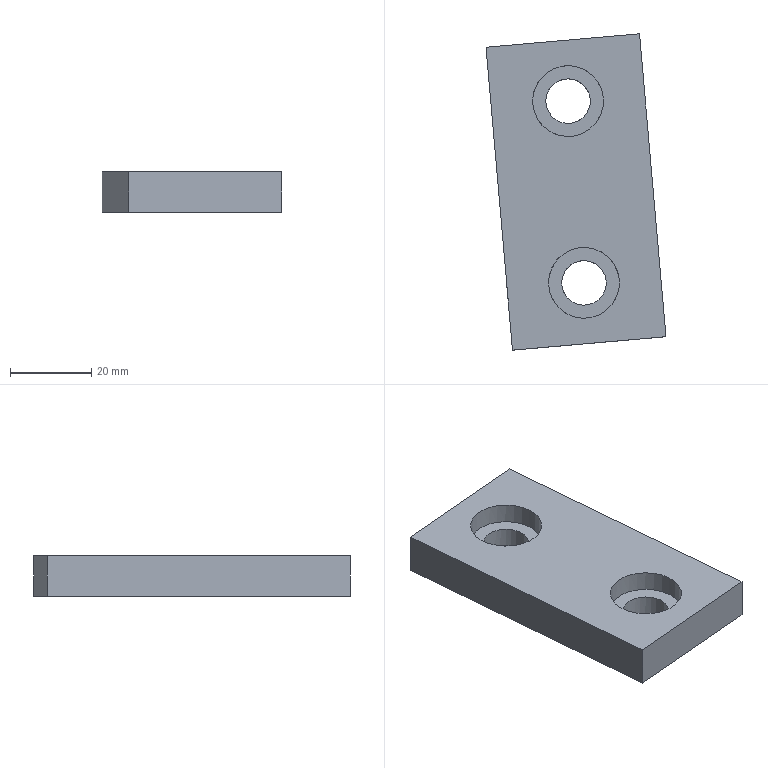Part | NX | features solid 2 | 1 solid | 12 faces | box 44.392 x 78.027 x 10 mm | volume 25144 mm3 | plane 8 | cylinder 4 | commonest cylinder face diameters 11 x2 17.5 x2
STEP:
#1=CARTESIAN_POINT('',(788.744,651.222,-208.));
#2=VERTEX_POINT('',#1);
#3=CARTESIAN_POINT('',(788.744,651.222,-218.));
#4=VERTEX_POINT('',#3);
#5=CARTESIAN_POINT('',(788.744,651.222,-208.));
#6=DIRECTION('',(0.,0.,-1.));
#7=VECTOR('',#6,1000.);
#8=LINE('',#5,#7);
#9=EDGE_CURVE('',#2,#4,#8,.T.);
#10=ORIENTED_EDGE('',*,*,#9,.F.);
#11=CARTESIAN_POINT('',(750.888,647.91,-208.));
#12=VERTEX_POINT('',#11);
#13=CARTESIAN_POINT('',(769.816,649.566,-208.));
#14=DIRECTION('',(0.9962,0.08716,0.));
#15=VECTOR('',#14,1000.);
#16=LINE('',#13,#15);
#17=EDGE_CURVE('',#12,#2,#16,.T.);
#18=ORIENTED_EDGE('',*,*,#17,.F.);
#19=CARTESIAN_POINT('',(750.888,647.91,-218.));
#20=VERTEX_POINT('',#19);
#21=CARTESIAN_POINT('',(750.888,647.91,-208.));
#22=DIRECTION('',(0.,0.,1.));
#23=VECTOR('',#22,1000.);
#24=LINE('',#21,#23);
#25=EDGE_CURVE('',#20,#12,#24,.T.);
#26=ORIENTED_EDGE('',*,*,#25,.F.);
#27=CARTESIAN_POINT('',(769.816,649.566,-218.));
#28=DIRECTION('',(-0.9962,-0.08716,0.));
#29=VECTOR('',#28,1000.);
#30=LINE('',#27,#29);
#31=EDGE_CURVE('',#4,#20,#30,.T.);
#32=ORIENTED_EDGE('',*,*,#31,.F.);
#33=EDGE_LOOP('',(#10,#18,#26,#32));
#34=FACE_BOUND('',#33,.T.);
#35=CARTESIAN_POINT('',(769.816,649.566,-208.));
#36=DIRECTION('',(0.08716,-0.9962,0.));
#37=DIRECTION('',(0.,0.,1.));
#38=AXIS2_PLACEMENT_3D('',#35,#36,#37);
#39=PLANE('',#38);
#40=ADVANCED_FACE('',(#34),#39,.T.);
#41=CARTESIAN_POINT('',(782.207,725.936,-208.));
#42=VERTEX_POINT('',#41);
#43=CARTESIAN_POINT('',(782.207,725.936,-208.));
#44=DIRECTION('',(0.08716,-0.9962,0.));
#45=VECTOR('',#44,1000.);
#46=LINE('',#43,#45);
#47=EDGE_CURVE('',#42,#2,#46,.T.);
#48=ORIENTED_EDGE('',*,*,#47,.T.);
#49=ORIENTED_EDGE('',*,*,#9,.T.);
#50=CARTESIAN_POINT('',(782.207,725.936,-218.));
#51=VERTEX_POINT('',#50);
#52=CARTESIAN_POINT('',(782.207,725.936,-218.));
#53=DIRECTION('',(0.08716,-0.9962,0.));
#54=VECTOR('',#53,1000.);
#55=LINE('',#52,#54);
#56=EDGE_CURVE('',#51,#4,#55,.T.);
#57=ORIENTED_EDGE('',*,*,#56,.F.);
#58=CARTESIAN_POINT('',(782.207,725.936,-208.));
#59=DIRECTION('',(0.,0.,1.));
#60=VECTOR('',#59,1000.);
#61=LINE('',#58,#60);
#62=EDGE_CURVE('',#51,#42,#61,.T.);
#63=ORIENTED_EDGE('',*,*,#62,.T.);
#64=EDGE_LOOP('',(#48,#49,#57,#63));
#65=FACE_BOUND('',#64,.T.);
#66=CARTESIAN_POINT('',(782.207,725.936,-208.));
#67=DIRECTION('',(0.9962,0.08716,0.));
#68=DIRECTION('',(-0.08716,0.9962,0.));
#69=AXIS2_PLACEMENT_3D('',#66,#67,#68);
#70=PLANE('',#69);
#71=ADVANCED_FACE('',(#65),#70,.T.);
#72=CARTESIAN_POINT('',(770.066,709.817,-218.));
#73=VERTEX_POINT('',#72);
#74=CARTESIAN_POINT('',(764.587,709.337,-218.));
#75=DIRECTION('',(0.,0.,1.));
#76=DIRECTION('',(0.9962,0.08716,0.));
#77=AXIS2_PLACEMENT_3D('',#74,#75,#76);
#78=CIRCLE('',#77,5.5);
#79=EDGE_CURVE('',#73,#73,#78,.T.);
#80=ORIENTED_EDGE('',*,*,#79,.T.);
#81=EDGE_LOOP('',(#80));
#82=FACE_BOUND('',#81,.T.);
#83=CARTESIAN_POINT('',(773.988,664.988,-218.));
#84=VERTEX_POINT('',#83);
#85=CARTESIAN_POINT('',(768.509,664.509,-218.));
#86=DIRECTION('',(0.,0.,1.));
#87=DIRECTION('',(0.9962,0.08716,0.));
#88=AXIS2_PLACEMENT_3D('',#85,#86,#87);
#89=CIRCLE('',#88,5.5);
#90=EDGE_CURVE('',#84,#84,#89,.T.);
#91=ORIENTED_EDGE('',*,*,#90,.T.);
#92=EDGE_LOOP('',(#91));
#93=FACE_BOUND('',#92,.T.);
#94=ORIENTED_EDGE('',*,*,#56,.T.);
#95=ORIENTED_EDGE('',*,*,#31,.T.);
#96=CARTESIAN_POINT('',(744.352,722.624,-218.));
#97=VERTEX_POINT('',#96);
#98=CARTESIAN_POINT('',(744.352,722.624,-218.));
#99=DIRECTION('',(0.08716,-0.9962,0.));
#100=VECTOR('',#99,1000.);
#101=LINE('',#98,#100);
#102=EDGE_CURVE('',#97,#20,#101,.T.);
#103=ORIENTED_EDGE('',*,*,#102,.F.);
#104=CARTESIAN_POINT('',(763.279,724.28,-218.));
#105=DIRECTION('',(0.9962,0.08716,0.));
#106=VECTOR('',#105,1000.);
#107=LINE('',#104,#106);
#108=EDGE_CURVE('',#97,#51,#107,.T.);
#109=ORIENTED_EDGE('',*,*,#108,.T.);
#110=EDGE_LOOP('',(#94,#95,#103,#109));
#111=FACE_BOUND('',#110,.T.);
#112=CARTESIAN_POINT('',(763.279,724.28,-218.));
#113=DIRECTION('',(0.,0.,-1.));
#114=DIRECTION('',(0.08716,-0.9962,0.));
#115=AXIS2_PLACEMENT_3D('',#112,#113,#114);
#116=PLANE('',#115);
#117=ADVANCED_FACE('',(#82,#93,#111),#116,.T.);
#118=ORIENTED_EDGE('',*,*,#102,.T.);
#119=ORIENTED_EDGE('',*,*,#25,.T.);
#120=CARTESIAN_POINT('',(744.352,722.624,-208.));
#121=VERTEX_POINT('',#120);
#122=CARTESIAN_POINT('',(744.352,722.624,-208.));
#123=DIRECTION('',(0.08716,-0.9962,0.));
#124=VECTOR('',#123,1000.);
#125=LINE('',#122,#124);
#126=EDGE_CURVE('',#121,#12,#125,.T.);
#127=ORIENTED_EDGE('',*,*,#126,.F.);
#128=CARTESIAN_POINT('',(744.352,722.624,-208.));
#129=DIRECTION('',(0.,0.,-1.));
#130=VECTOR('',#129,1000.);
#131=LINE('',#128,#130);
#132=EDGE_CURVE('',#121,#97,#131,.T.);
#133=ORIENTED_EDGE('',*,*,#132,.T.);
#134=EDGE_LOOP('',(#118,#119,#127,#133));
#135=FACE_BOUND('',#134,.T.);
#136=CARTESIAN_POINT('',(744.352,722.624,-208.));
#137=DIRECTION('',(-0.9962,-0.08716,0.));
#138=DIRECTION('',(0.08716,-0.9962,0.));
#139=AXIS2_PLACEMENT_3D('',#136,#137,#138);
#140=PLANE('',#139);
#141=ADVANCED_FACE('',(#135),#140,.T.);
#142=CARTESIAN_POINT('',(763.279,724.28,-208.));
#143=DIRECTION('',(-0.9962,-0.08716,0.));
#144=VECTOR('',#143,1000.);
#145=LINE('',#142,#144);
#146=EDGE_CURVE('',#42,#121,#145,.T.);
#147=ORIENTED_EDGE('',*,*,#146,.F.);
#148=ORIENTED_EDGE('',*,*,#62,.F.);
#149=ORIENTED_EDGE('',*,*,#108,.F.);
#150=ORIENTED_EDGE('',*,*,#132,.F.);
#151=EDGE_LOOP('',(#147,#148,#149,#150));
#152=FACE_BOUND('',#151,.T.);
#153=CARTESIAN_POINT('',(763.279,724.28,-208.));
#154=DIRECTION('',(-0.08716,0.9962,0.));
#155=DIRECTION('',(0.,0.,-1.));
#156=AXIS2_PLACEMENT_3D('',#153,#154,#155);
#157=PLANE('',#156);
#158=ADVANCED_FACE('',(#152),#157,.T.);
#159=CARTESIAN_POINT('',(755.837,709.337,-208.));
#160=VERTEX_POINT('',#159);
#161=CARTESIAN_POINT('',(764.587,709.337,-208.));
#162=DIRECTION('',(0.,0.,-1.));
#163=DIRECTION('',(-1.,0.,0.));
#164=AXIS2_PLACEMENT_3D('',#161,#162,#163);
#165=CIRCLE('',#164,8.75);
#166=EDGE_CURVE('',#160,#160,#165,.T.);
#167=ORIENTED_EDGE('',*,*,#166,.T.);
#168=EDGE_LOOP('',(#167));
#169=FACE_BOUND('',#168,.T.);
#170=CARTESIAN_POINT('',(759.759,664.509,-208.));
#171=VERTEX_POINT('',#170);
#172=CARTESIAN_POINT('',(768.509,664.509,-208.));
#173=DIRECTION('',(0.,0.,-1.));
#174=DIRECTION('',(-1.,0.,0.));
#175=AXIS2_PLACEMENT_3D('',#172,#173,#174);
#176=CIRCLE('',#175,8.75);
#177=EDGE_CURVE('',#171,#171,#176,.T.);
#178=ORIENTED_EDGE('',*,*,#177,.T.);
#179=EDGE_LOOP('',(#178));
#180=FACE_BOUND('',#179,.T.);
#181=ORIENTED_EDGE('',*,*,#146,.T.);
#182=ORIENTED_EDGE('',*,*,#126,.T.);
#183=ORIENTED_EDGE('',*,*,#17,.T.);
#184=ORIENTED_EDGE('',*,*,#47,.F.);
#185=EDGE_LOOP('',(#181,#182,#183,#184));
#186=FACE_BOUND('',#185,.T.);
#187=CARTESIAN_POINT('',(763.279,724.28,-208.));
#188=DIRECTION('',(0.,0.,1.));
#189=DIRECTION('',(-0.08716,0.9962,0.));
#190=AXIS2_PLACEMENT_3D('',#187,#188,#189);
#191=PLANE('',#190);
#192=ADVANCED_FACE('',(#169,#180,#186),#191,.T.);
#193=CARTESIAN_POINT('',(763.009,664.509,-213.));
#194=VERTEX_POINT('',#193);
#195=CARTESIAN_POINT('',(768.509,664.509,-213.));
#196=DIRECTION('',(0.,0.,-1.));
#197=DIRECTION('',(-1.,0.,0.));
#198=AXIS2_PLACEMENT_3D('',#195,#196,#197);
#199=CIRCLE('',#198,5.5);
#200=EDGE_CURVE('',#194,#194,#199,.F.);
#201=ORIENTED_EDGE('',*,*,#200,.T.);
#202=EDGE_LOOP('',(#201));
#203=FACE_BOUND('',#202,.T.);
#204=ORIENTED_EDGE('',*,*,#90,.F.);
#205=EDGE_LOOP('',(#204));
#206=FACE_BOUND('',#205,.T.);
#207=CARTESIAN_POINT('',(768.509,664.509,-218.));
#208=DIRECTION('',(0.,0.,1.));
#209=DIRECTION('',(0.9962,0.08716,0.));
#210=AXIS2_PLACEMENT_3D('',#207,#208,#209);
#211=CYLINDRICAL_SURFACE('',#210,5.5);
#212=ADVANCED_FACE('',(#203,#206),#211,.F.);
#213=CARTESIAN_POINT('',(777.225,665.271,-213.));
#214=VERTEX_POINT('',#213);
#215=CARTESIAN_POINT('',(768.509,664.509,-213.));
#216=DIRECTION('',(0.,0.,1.));
#217=DIRECTION('',(0.9962,0.08716,0.));
#218=AXIS2_PLACEMENT_3D('',#215,#216,#217);
#219=CIRCLE('',#218,8.75);
#220=EDGE_CURVE('',#214,#214,#219,.T.);
#221=ORIENTED_EDGE('',*,*,#220,.T.);
#222=EDGE_LOOP('',(#221));
#223=FACE_BOUND('',#222,.T.);
#224=ORIENTED_EDGE('',*,*,#200,.F.);
#225=EDGE_LOOP('',(#224));
#226=FACE_BOUND('',#225,.T.);
#227=CARTESIAN_POINT('',(768.509,664.509,-213.));
#228=DIRECTION('',(0.,0.,-1.));
#229=DIRECTION('',(-0.9962,-0.08716,0.));
#230=AXIS2_PLACEMENT_3D('',#227,#228,#229);
#231=PLANE('',#230);
#232=ADVANCED_FACE('',(#223,#226),#231,.F.);
#233=ORIENTED_EDGE('',*,*,#177,.F.);
#234=EDGE_LOOP('',(#233));
#235=FACE_BOUND('',#234,.T.);
#236=ORIENTED_EDGE('',*,*,#220,.F.);
#237=EDGE_LOOP('',(#236));
#238=FACE_BOUND('',#237,.T.);
#239=CARTESIAN_POINT('',(768.509,664.509,-213.));
#240=DIRECTION('',(0.,0.,1.));
#241=DIRECTION('',(0.9962,0.08716,0.));
#242=AXIS2_PLACEMENT_3D('',#239,#240,#241);
#243=CYLINDRICAL_SURFACE('',#242,8.75);
#244=ADVANCED_FACE('',(#235,#238),#243,.F.);
#245=CARTESIAN_POINT('',(759.087,709.337,-213.));
#246=VERTEX_POINT('',#245);
#247=CARTESIAN_POINT('',(764.587,709.337,-213.));
#248=DIRECTION('',(0.,0.,-1.));
#249=DIRECTION('',(-1.,0.,0.));
#250=AXIS2_PLACEMENT_3D('',#247,#248,#249);
#251=CIRCLE('',#250,5.5);
#252=EDGE_CURVE('',#246,#246,#251,.F.);
#253=ORIENTED_EDGE('',*,*,#252,.T.);
#254=EDGE_LOOP('',(#253));
#255=FACE_BOUND('',#254,.T.);
#256=ORIENTED_EDGE('',*,*,#79,.F.);
#257=EDGE_LOOP('',(#256));
#258=FACE_BOUND('',#257,.T.);
#259=CARTESIAN_POINT('',(764.587,709.337,-218.));
#260=DIRECTION('',(0.,0.,1.));
#261=DIRECTION('',(0.9962,0.08716,0.));
#262=AXIS2_PLACEMENT_3D('',#259,#260,#261);
#263=CYLINDRICAL_SURFACE('',#262,5.5);
#264=ADVANCED_FACE('',(#255,#258),#263,.F.);
#265=CARTESIAN_POINT('',(773.303,710.1,-213.));
#266=VERTEX_POINT('',#265);
#267=CARTESIAN_POINT('',(764.587,709.337,-213.));
#268=DIRECTION('',(0.,0.,1.));
#269=DIRECTION('',(0.9962,0.08716,0.));
#270=AXIS2_PLACEMENT_3D('',#267,#268,#269);
#271=CIRCLE('',#270,8.75);
#272=EDGE_CURVE('',#266,#266,#271,.T.);
#273=ORIENTED_EDGE('',*,*,#272,.T.);
#274=EDGE_LOOP('',(#273));
#275=FACE_BOUND('',#274,.T.);
#276=ORIENTED_EDGE('',*,*,#252,.F.);
#277=EDGE_LOOP('',(#276));
#278=FACE_BOUND('',#277,.T.);
#279=CARTESIAN_POINT('',(764.587,709.337,-213.));
#280=DIRECTION('',(0.,0.,-1.));
#281=DIRECTION('',(-0.9962,-0.08716,0.));
#282=AXIS2_PLACEMENT_3D('',#279,#280,#281);
#283=PLANE('',#282);
#284=ADVANCED_FACE('',(#275,#278),#283,.F.);
#285=ORIENTED_EDGE('',*,*,#166,.F.);
#286=EDGE_LOOP('',(#285));
#287=FACE_BOUND('',#286,.T.);
#288=ORIENTED_EDGE('',*,*,#272,.F.);
#289=EDGE_LOOP('',(#288));
#290=FACE_BOUND('',#289,.T.);
#291=CARTESIAN_POINT('',(764.587,709.337,-213.));
#292=DIRECTION('',(0.,0.,1.));
#293=DIRECTION('',(0.9962,0.08716,0.));
#294=AXIS2_PLACEMENT_3D('',#291,#292,#293);
#295=CYLINDRICAL_SURFACE('',#294,8.75);
#296=ADVANCED_FACE('',(#287,#290),#295,.F.);
#297=CLOSED_SHELL('',(#40,#71,#117,#141,#158,#192,#212,#232,#244,#264,#284,#296));
#298=MANIFOLD_SOLID_BREP('',#297);
#299=(LENGTH_UNIT()NAMED_UNIT(*)SI_UNIT(.MILLI.,.METRE.));
#300=UNCERTAINTY_MEASURE_WITH_UNIT(LENGTH_MEASURE(0.00001),#299,'','');
#301=(NAMED_UNIT(*)PLANE_ANGLE_UNIT()SI_UNIT($,.RADIAN.));
#302=(NAMED_UNIT(*)SI_UNIT($,.STERADIAN.)SOLID_ANGLE_UNIT());
#303=(GEOMETRIC_REPRESENTATION_CONTEXT(3)GLOBAL_UNCERTAINTY_ASSIGNED_CONTEXT((#300))GLOBAL_UNIT_ASSIGNED_CONTEXT((#299,#301,#302))REPRESENTATION_CONTEXT('',''));
#304=ADVANCED_BREP_SHAPE_REPRESENTATION('',(#298),#303);